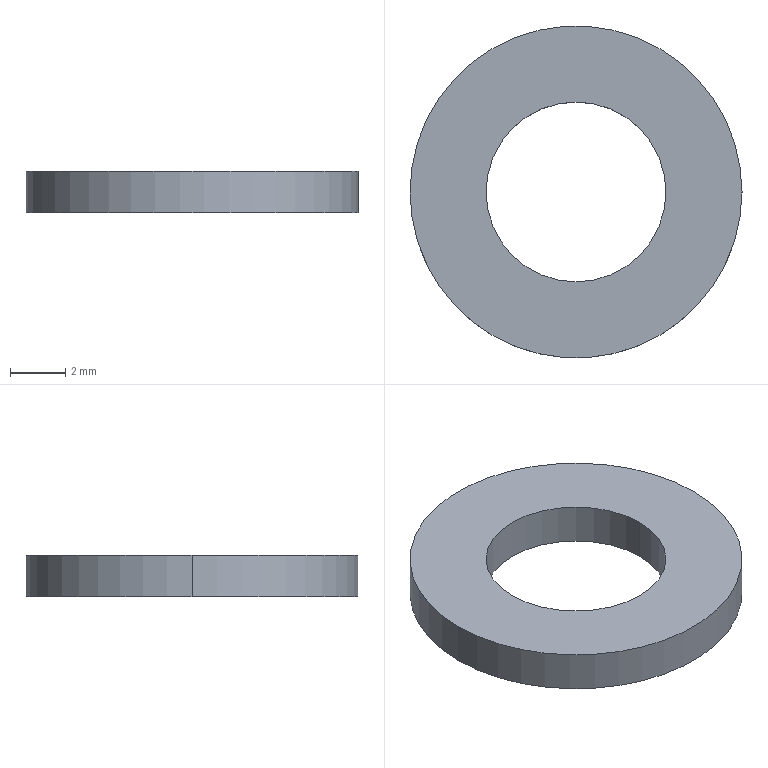Part | STEP file | 6mm stainless steel flat washer | 1 solid | 6 faces | box 12 x 12 x 1.5 mm | volume 119.871 mm3 | cylinder 4 | plane 2 | commonest cylinder face diameters 6.5 x2 12 x2
STEP:
#1=CARTESIAN_POINT('',(0.,0.,0.));
#2=DIRECTION('',(0.,0.,1.));
#3=DIRECTION('',(1.,0.,0.));
#4=AXIS2_PLACEMENT_3D('',#1,#2,#3);
#5=CARTESIAN_POINT('',(-3.25,0.,1.5));
#6=VERTEX_POINT('',#5);
#7=CARTESIAN_POINT('',(-3.25,0.,0.));
#8=VERTEX_POINT('',#7);
#9=CARTESIAN_POINT('',(-3.25,0.,1.5));
#10=DIRECTION('',(0.,0.,-1.));
#11=VECTOR('',#10,1.);
#12=LINE('',#9,#11);
#13=CARTESIAN_POINT('',(0.,0.,1.5));
#14=DIRECTION('',(0.,0.,-1.));
#15=DIRECTION('',(-1.,0.,0.));
#16=AXIS2_PLACEMENT_3D('',#13,#14,#15);
#17=CYLINDRICAL_SURFACE('',#16,3.25);
#18=CARTESIAN_POINT('',(6.283,0.));
#19=DIRECTION('',(0.,1.));
#20=VECTOR('',#19,1.);
#21=LINE('',#18,#20);
#22=(GEOMETRIC_REPRESENTATION_CONTEXT(2)PARAMETRIC_REPRESENTATION_CONTEXT()REPRESENTATION_CONTEXT('',''));
#23=DEFINITIONAL_REPRESENTATION('',(#21),#22);
#24=PCURVE('',#17,#23);
#25=CARTESIAN_POINT('',(0.,0.,1.5));
#26=DIRECTION('',(0.,0.,-1.));
#27=DIRECTION('',(-1.,0.,0.));
#28=AXIS2_PLACEMENT_3D('',#25,#26,#27);
#29=CYLINDRICAL_SURFACE('',#28,3.25);
#30=CARTESIAN_POINT('',(0.,0.));
#31=DIRECTION('',(0.,1.));
#32=VECTOR('',#31,1.);
#33=LINE('',#30,#32);
#34=(GEOMETRIC_REPRESENTATION_CONTEXT(2)PARAMETRIC_REPRESENTATION_CONTEXT()REPRESENTATION_CONTEXT('',''));
#35=DEFINITIONAL_REPRESENTATION('',(#33),#34);
#36=PCURVE('',#29,#35);
#37=SURFACE_CURVE('',#12,(#24,#36),.PCURVE_S1.);
#38=EDGE_CURVE('',#6,#8,#37,.T.);
#39=ORIENTED_EDGE('',*,*,#38,.T.);
#40=CARTESIAN_POINT('',(3.25,0.,0.));
#41=VERTEX_POINT('',#40);
#42=CARTESIAN_POINT('',(0.,0.,0.));
#43=DIRECTION('',(0.,0.,1.));
#44=DIRECTION('',(1.,0.,0.));
#45=AXIS2_PLACEMENT_3D('',#42,#43,#44);
#46=CIRCLE('',#45,3.25);
#47=CARTESIAN_POINT('',(9.425,1.5));
#48=DIRECTION('',(-1.,0.));
#49=VECTOR('',#48,1.);
#50=LINE('',#47,#49);
#51=(GEOMETRIC_REPRESENTATION_CONTEXT(2)PARAMETRIC_REPRESENTATION_CONTEXT()REPRESENTATION_CONTEXT('',''));
#52=DEFINITIONAL_REPRESENTATION('',(#50),#51);
#53=PCURVE('',#17,#52);
#54=CARTESIAN_POINT('',(0.,0.,0.));
#55=DIRECTION('',(0.,0.,1.));
#56=DIRECTION('',(1.,0.,0.));
#57=AXIS2_PLACEMENT_3D('',#54,#55,#56);
#58=PLANE('',#57);
#59=CARTESIAN_POINT('',(0.,0.));
#60=DIRECTION('',(1.,0.));
#61=AXIS2_PLACEMENT_2D('',#59,#60);
#62=CIRCLE('',#61,3.25);
#63=(GEOMETRIC_REPRESENTATION_CONTEXT(2)PARAMETRIC_REPRESENTATION_CONTEXT()REPRESENTATION_CONTEXT('',''));
#64=DEFINITIONAL_REPRESENTATION('',(#62),#63);
#65=PCURVE('',#58,#64);
#66=SURFACE_CURVE('',#46,(#53,#65),.PCURVE_S1.);
#67=EDGE_CURVE('',#8,#41,#66,.T.);
#68=ORIENTED_EDGE('',*,*,#67,.T.);
#69=CARTESIAN_POINT('',(3.25,0.,1.5));
#70=VERTEX_POINT('',#69);
#71=CARTESIAN_POINT('',(3.25,0.,1.5));
#72=DIRECTION('',(0.,0.,-1.));
#73=VECTOR('',#72,1.);
#74=LINE('',#71,#73);
#75=CARTESIAN_POINT('',(3.142,0.));
#76=DIRECTION('',(0.,1.));
#77=VECTOR('',#76,1.);
#78=LINE('',#75,#77);
#79=(GEOMETRIC_REPRESENTATION_CONTEXT(2)PARAMETRIC_REPRESENTATION_CONTEXT()REPRESENTATION_CONTEXT('',''));
#80=DEFINITIONAL_REPRESENTATION('',(#78),#79);
#81=PCURVE('',#17,#80);
#82=CARTESIAN_POINT('',(3.142,0.));
#83=DIRECTION('',(0.,1.));
#84=VECTOR('',#83,1.);
#85=LINE('',#82,#84);
#86=(GEOMETRIC_REPRESENTATION_CONTEXT(2)PARAMETRIC_REPRESENTATION_CONTEXT()REPRESENTATION_CONTEXT('',''));
#87=DEFINITIONAL_REPRESENTATION('',(#85),#86);
#88=PCURVE('',#29,#87);
#89=SURFACE_CURVE('',#74,(#81,#88),.PCURVE_S1.);
#90=EDGE_CURVE('',#70,#41,#89,.T.);
#91=ORIENTED_EDGE('',*,*,#90,.F.);
#92=CARTESIAN_POINT('',(0.,0.,1.5));
#93=DIRECTION('',(0.,0.,1.));
#94=DIRECTION('',(1.,0.,0.));
#95=AXIS2_PLACEMENT_3D('',#92,#93,#94);
#96=CIRCLE('',#95,3.25);
#97=CARTESIAN_POINT('',(9.425,0.));
#98=DIRECTION('',(-1.,0.));
#99=VECTOR('',#98,1.);
#100=LINE('',#97,#99);
#101=(GEOMETRIC_REPRESENTATION_CONTEXT(2)PARAMETRIC_REPRESENTATION_CONTEXT()REPRESENTATION_CONTEXT('',''));
#102=DEFINITIONAL_REPRESENTATION('',(#100),#101);
#103=PCURVE('',#17,#102);
#104=CARTESIAN_POINT('',(0.,0.,1.5));
#105=DIRECTION('',(0.,0.,1.));
#106=DIRECTION('',(1.,0.,0.));
#107=AXIS2_PLACEMENT_3D('',#104,#105,#106);
#108=PLANE('',#107);
#109=CARTESIAN_POINT('',(0.,0.));
#110=DIRECTION('',(1.,0.));
#111=AXIS2_PLACEMENT_2D('',#109,#110);
#112=CIRCLE('',#111,3.25);
#113=(GEOMETRIC_REPRESENTATION_CONTEXT(2)PARAMETRIC_REPRESENTATION_CONTEXT()REPRESENTATION_CONTEXT('',''));
#114=DEFINITIONAL_REPRESENTATION('',(#112),#113);
#115=PCURVE('',#108,#114);
#116=SURFACE_CURVE('',#96,(#103,#115),.PCURVE_S1.);
#117=EDGE_CURVE('',#6,#70,#116,.T.);
#118=ORIENTED_EDGE('',*,*,#117,.F.);
#119=EDGE_LOOP('',(#39,#68,#91,#118));
#120=FACE_BOUND('',#119,.F.);
#121=ADVANCED_FACE('',(#120),#17,.F.);
#122=CARTESIAN_POINT('',(6.,0.,1.5));
#123=VERTEX_POINT('',#122);
#124=CARTESIAN_POINT('',(-6.,0.,1.5));
#125=VERTEX_POINT('',#124);
#126=CARTESIAN_POINT('',(0.,0.,1.5));
#127=DIRECTION('',(0.,0.,1.));
#128=DIRECTION('',(1.,0.,0.));
#129=AXIS2_PLACEMENT_3D('',#126,#127,#128);
#130=CIRCLE('',#129,6.);
#131=CARTESIAN_POINT('',(0.,0.,1.5));
#132=DIRECTION('',(0.,0.,-1.));
#133=DIRECTION('',(-1.,0.,0.));
#134=AXIS2_PLACEMENT_3D('',#131,#132,#133);
#135=CYLINDRICAL_SURFACE('',#134,6.);
#136=CARTESIAN_POINT('',(3.142,0.));
#137=DIRECTION('',(-1.,0.));
#138=VECTOR('',#137,1.);
#139=LINE('',#136,#138);
#140=(GEOMETRIC_REPRESENTATION_CONTEXT(2)PARAMETRIC_REPRESENTATION_CONTEXT()REPRESENTATION_CONTEXT('',''));
#141=DEFINITIONAL_REPRESENTATION('',(#139),#140);
#142=PCURVE('',#135,#141);
#143=CARTESIAN_POINT('',(0.,0.));
#144=DIRECTION('',(1.,0.));
#145=AXIS2_PLACEMENT_2D('',#143,#144);
#146=CIRCLE('',#145,6.);
#147=(GEOMETRIC_REPRESENTATION_CONTEXT(2)PARAMETRIC_REPRESENTATION_CONTEXT()REPRESENTATION_CONTEXT('',''));
#148=DEFINITIONAL_REPRESENTATION('',(#146),#147);
#149=PCURVE('',#108,#148);
#150=SURFACE_CURVE('',#130,(#142,#149),.PCURVE_S1.);
#151=EDGE_CURVE('',#123,#125,#150,.T.);
#152=ORIENTED_EDGE('',*,*,#151,.F.);
#153=CARTESIAN_POINT('',(6.,0.,0.));
#154=VERTEX_POINT('',#153);
#155=CARTESIAN_POINT('',(6.,0.,1.5));
#156=DIRECTION('',(0.,0.,-1.));
#157=VECTOR('',#156,1.);
#158=LINE('',#155,#157);
#159=CARTESIAN_POINT('',(3.142,0.));
#160=DIRECTION('',(0.,1.));
#161=VECTOR('',#160,1.);
#162=LINE('',#159,#161);
#163=(GEOMETRIC_REPRESENTATION_CONTEXT(2)PARAMETRIC_REPRESENTATION_CONTEXT()REPRESENTATION_CONTEXT('',''));
#164=DEFINITIONAL_REPRESENTATION('',(#162),#163);
#165=PCURVE('',#135,#164);
#166=CARTESIAN_POINT('',(0.,0.,1.5));
#167=DIRECTION('',(0.,0.,-1.));
#168=DIRECTION('',(-1.,0.,0.));
#169=AXIS2_PLACEMENT_3D('',#166,#167,#168);
#170=CYLINDRICAL_SURFACE('',#169,6.);
#171=CARTESIAN_POINT('',(3.142,0.));
#172=DIRECTION('',(0.,1.));
#173=VECTOR('',#172,1.);
#174=LINE('',#171,#173);
#175=(GEOMETRIC_REPRESENTATION_CONTEXT(2)PARAMETRIC_REPRESENTATION_CONTEXT()REPRESENTATION_CONTEXT('',''));
#176=DEFINITIONAL_REPRESENTATION('',(#174),#175);
#177=PCURVE('',#170,#176);
#178=SURFACE_CURVE('',#158,(#165,#177),.PCURVE_S1.);
#179=EDGE_CURVE('',#123,#154,#178,.T.);
#180=ORIENTED_EDGE('',*,*,#179,.T.);
#181=CARTESIAN_POINT('',(-6.,0.,0.));
#182=VERTEX_POINT('',#181);
#183=CARTESIAN_POINT('',(0.,0.,0.));
#184=DIRECTION('',(0.,0.,1.));
#185=DIRECTION('',(1.,0.,0.));
#186=AXIS2_PLACEMENT_3D('',#183,#184,#185);
#187=CIRCLE('',#186,6.);
#188=CARTESIAN_POINT('',(3.142,1.5));
#189=DIRECTION('',(-1.,0.));
#190=VECTOR('',#189,1.);
#191=LINE('',#188,#190);
#192=(GEOMETRIC_REPRESENTATION_CONTEXT(2)PARAMETRIC_REPRESENTATION_CONTEXT()REPRESENTATION_CONTEXT('',''));
#193=DEFINITIONAL_REPRESENTATION('',(#191),#192);
#194=PCURVE('',#135,#193);
#195=CARTESIAN_POINT('',(0.,0.));
#196=DIRECTION('',(1.,0.));
#197=AXIS2_PLACEMENT_2D('',#195,#196);
#198=CIRCLE('',#197,6.);
#199=(GEOMETRIC_REPRESENTATION_CONTEXT(2)PARAMETRIC_REPRESENTATION_CONTEXT()REPRESENTATION_CONTEXT('',''));
#200=DEFINITIONAL_REPRESENTATION('',(#198),#199);
#201=PCURVE('',#58,#200);
#202=SURFACE_CURVE('',#187,(#194,#201),.PCURVE_S1.);
#203=EDGE_CURVE('',#154,#182,#202,.T.);
#204=ORIENTED_EDGE('',*,*,#203,.T.);
#205=CARTESIAN_POINT('',(-6.,0.,1.5));
#206=DIRECTION('',(0.,0.,-1.));
#207=VECTOR('',#206,1.);
#208=LINE('',#205,#207);
#209=CARTESIAN_POINT('',(0.,0.));
#210=DIRECTION('',(0.,1.));
#211=VECTOR('',#210,1.);
#212=LINE('',#209,#211);
#213=(GEOMETRIC_REPRESENTATION_CONTEXT(2)PARAMETRIC_REPRESENTATION_CONTEXT()REPRESENTATION_CONTEXT('',''));
#214=DEFINITIONAL_REPRESENTATION('',(#212),#213);
#215=PCURVE('',#135,#214);
#216=CARTESIAN_POINT('',(6.283,0.));
#217=DIRECTION('',(0.,1.));
#218=VECTOR('',#217,1.);
#219=LINE('',#216,#218);
#220=(GEOMETRIC_REPRESENTATION_CONTEXT(2)PARAMETRIC_REPRESENTATION_CONTEXT()REPRESENTATION_CONTEXT('',''));
#221=DEFINITIONAL_REPRESENTATION('',(#219),#220);
#222=PCURVE('',#170,#221);
#223=SURFACE_CURVE('',#208,(#215,#222),.PCURVE_S1.);
#224=EDGE_CURVE('',#125,#182,#223,.T.);
#225=ORIENTED_EDGE('',*,*,#224,.F.);
#226=EDGE_LOOP('',(#152,#180,#204,#225));
#227=FACE_BOUND('',#226,.T.);
#228=ADVANCED_FACE('',(#227),#135,.T.);
#229=CARTESIAN_POINT('',(0.,0.,1.5));
#230=DIRECTION('',(0.,0.,1.));
#231=DIRECTION('',(1.,0.,0.));
#232=AXIS2_PLACEMENT_3D('',#229,#230,#231);
#233=CIRCLE('',#232,6.);
#234=CARTESIAN_POINT('',(0.,0.));
#235=DIRECTION('',(1.,0.));
#236=AXIS2_PLACEMENT_2D('',#234,#235);
#237=CIRCLE('',#236,6.);
#238=(GEOMETRIC_REPRESENTATION_CONTEXT(2)PARAMETRIC_REPRESENTATION_CONTEXT()REPRESENTATION_CONTEXT('',''));
#239=DEFINITIONAL_REPRESENTATION('',(#237),#238);
#240=PCURVE('',#108,#239);
#241=CARTESIAN_POINT('',(9.425,0.));
#242=DIRECTION('',(-1.,0.));
#243=VECTOR('',#242,1.);
#244=LINE('',#241,#243);
#245=(GEOMETRIC_REPRESENTATION_CONTEXT(2)PARAMETRIC_REPRESENTATION_CONTEXT()REPRESENTATION_CONTEXT('',''));
#246=DEFINITIONAL_REPRESENTATION('',(#244),#245);
#247=PCURVE('',#170,#246);
#248=SURFACE_CURVE('',#233,(#240,#247),.PCURVE_S1.);
#249=EDGE_CURVE('',#125,#123,#248,.T.);
#250=ORIENTED_EDGE('',*,*,#249,.T.);
#251=ORIENTED_EDGE('',*,*,#151,.T.);
#252=EDGE_LOOP('',(#250,#251));
#253=FACE_BOUND('',#252,.T.);
#254=ORIENTED_EDGE('',*,*,#117,.F.);
#255=CARTESIAN_POINT('',(0.,0.,1.5));
#256=DIRECTION('',(0.,0.,1.));
#257=DIRECTION('',(1.,0.,0.));
#258=AXIS2_PLACEMENT_3D('',#255,#256,#257);
#259=CIRCLE('',#258,3.25);
#260=CARTESIAN_POINT('',(0.,0.));
#261=DIRECTION('',(1.,0.));
#262=AXIS2_PLACEMENT_2D('',#260,#261);
#263=CIRCLE('',#262,3.25);
#264=(GEOMETRIC_REPRESENTATION_CONTEXT(2)PARAMETRIC_REPRESENTATION_CONTEXT()REPRESENTATION_CONTEXT('',''));
#265=DEFINITIONAL_REPRESENTATION('',(#263),#264);
#266=PCURVE('',#108,#265);
#267=CARTESIAN_POINT('',(3.142,0.));
#268=DIRECTION('',(-1.,0.));
#269=VECTOR('',#268,1.);
#270=LINE('',#267,#269);
#271=(GEOMETRIC_REPRESENTATION_CONTEXT(2)PARAMETRIC_REPRESENTATION_CONTEXT()REPRESENTATION_CONTEXT('',''));
#272=DEFINITIONAL_REPRESENTATION('',(#270),#271);
#273=PCURVE('',#29,#272);
#274=SURFACE_CURVE('',#259,(#266,#273),.PCURVE_S1.);
#275=EDGE_CURVE('',#70,#6,#274,.T.);
#276=ORIENTED_EDGE('',*,*,#275,.F.);
#277=EDGE_LOOP('',(#254,#276));
#278=FACE_BOUND('',#277,.T.);
#279=ADVANCED_FACE('',(#253,#278),#108,.T.);
#280=CARTESIAN_POINT('',(0.,0.,0.));
#281=DIRECTION('',(0.,0.,1.));
#282=DIRECTION('',(1.,0.,0.));
#283=AXIS2_PLACEMENT_3D('',#280,#281,#282);
#284=CIRCLE('',#283,6.);
#285=CARTESIAN_POINT('',(0.,0.));
#286=DIRECTION('',(1.,0.));
#287=AXIS2_PLACEMENT_2D('',#285,#286);
#288=CIRCLE('',#287,6.);
#289=(GEOMETRIC_REPRESENTATION_CONTEXT(2)PARAMETRIC_REPRESENTATION_CONTEXT()REPRESENTATION_CONTEXT('',''));
#290=DEFINITIONAL_REPRESENTATION('',(#288),#289);
#291=PCURVE('',#58,#290);
#292=CARTESIAN_POINT('',(9.425,1.5));
#293=DIRECTION('',(-1.,0.));
#294=VECTOR('',#293,1.);
#295=LINE('',#292,#294);
#296=(GEOMETRIC_REPRESENTATION_CONTEXT(2)PARAMETRIC_REPRESENTATION_CONTEXT()REPRESENTATION_CONTEXT('',''));
#297=DEFINITIONAL_REPRESENTATION('',(#295),#296);
#298=PCURVE('',#170,#297);
#299=SURFACE_CURVE('',#284,(#291,#298),.PCURVE_S1.);
#300=EDGE_CURVE('',#182,#154,#299,.T.);
#301=ORIENTED_EDGE('',*,*,#300,.F.);
#302=ORIENTED_EDGE('',*,*,#203,.F.);
#303=EDGE_LOOP('',(#301,#302));
#304=FACE_BOUND('',#303,.T.);
#305=ORIENTED_EDGE('',*,*,#67,.T.);
#306=CARTESIAN_POINT('',(0.,0.,0.));
#307=DIRECTION('',(0.,0.,1.));
#308=DIRECTION('',(1.,0.,0.));
#309=AXIS2_PLACEMENT_3D('',#306,#307,#308);
#310=CIRCLE('',#309,3.25);
#311=CARTESIAN_POINT('',(0.,0.));
#312=DIRECTION('',(1.,0.));
#313=AXIS2_PLACEMENT_2D('',#311,#312);
#314=CIRCLE('',#313,3.25);
#315=(GEOMETRIC_REPRESENTATION_CONTEXT(2)PARAMETRIC_REPRESENTATION_CONTEXT()REPRESENTATION_CONTEXT('',''));
#316=DEFINITIONAL_REPRESENTATION('',(#314),#315);
#317=PCURVE('',#58,#316);
#318=CARTESIAN_POINT('',(3.142,1.5));
#319=DIRECTION('',(-1.,0.));
#320=VECTOR('',#319,1.);
#321=LINE('',#318,#320);
#322=(GEOMETRIC_REPRESENTATION_CONTEXT(2)PARAMETRIC_REPRESENTATION_CONTEXT()REPRESENTATION_CONTEXT('',''));
#323=DEFINITIONAL_REPRESENTATION('',(#321),#322);
#324=PCURVE('',#29,#323);
#325=SURFACE_CURVE('',#310,(#317,#324),.PCURVE_S1.);
#326=EDGE_CURVE('',#41,#8,#325,.T.);
#327=ORIENTED_EDGE('',*,*,#326,.T.);
#328=EDGE_LOOP('',(#305,#327));
#329=FACE_BOUND('',#328,.T.);
#330=ADVANCED_FACE('',(#304,#329),#58,.F.);
#331=ORIENTED_EDGE('',*,*,#179,.F.);
#332=ORIENTED_EDGE('',*,*,#249,.F.);
#333=ORIENTED_EDGE('',*,*,#224,.T.);
#334=ORIENTED_EDGE('',*,*,#300,.T.);
#335=EDGE_LOOP('',(#331,#332,#333,#334));
#336=FACE_BOUND('',#335,.T.);
#337=ADVANCED_FACE('',(#336),#170,.T.);
#338=ORIENTED_EDGE('',*,*,#326,.T.);
#339=ORIENTED_EDGE('',*,*,#38,.F.);
#340=ORIENTED_EDGE('',*,*,#275,.F.);
#341=ORIENTED_EDGE('',*,*,#90,.T.);
#342=EDGE_LOOP('',(#338,#339,#340,#341));
#343=FACE_BOUND('',#342,.F.);
#344=ADVANCED_FACE('',(#343),#29,.F.);
#345=CLOSED_SHELL('',(#121,#228,#279,#330,#337,#344));
#346=MANIFOLD_SOLID_BREP('',#345);
#347=(LENGTH_UNIT()NAMED_UNIT(*)SI_UNIT(.MILLI.,.METRE.));
#348=UNCERTAINTY_MEASURE_WITH_UNIT(LENGTH_MEASURE(0.0000001),#347,'','');
#349=(NAMED_UNIT(*)PLANE_ANGLE_UNIT()SI_UNIT($,.RADIAN.));
#350=(NAMED_UNIT(*)SI_UNIT($,.STERADIAN.)SOLID_ANGLE_UNIT());
#351=(GEOMETRIC_REPRESENTATION_CONTEXT(3)GLOBAL_UNCERTAINTY_ASSIGNED_CONTEXT((#348))GLOBAL_UNIT_ASSIGNED_CONTEXT((#347,#349,#350))REPRESENTATION_CONTEXT('',''));
#352=ADVANCED_BREP_SHAPE_REPRESENTATION('',(#4,#346),#351);